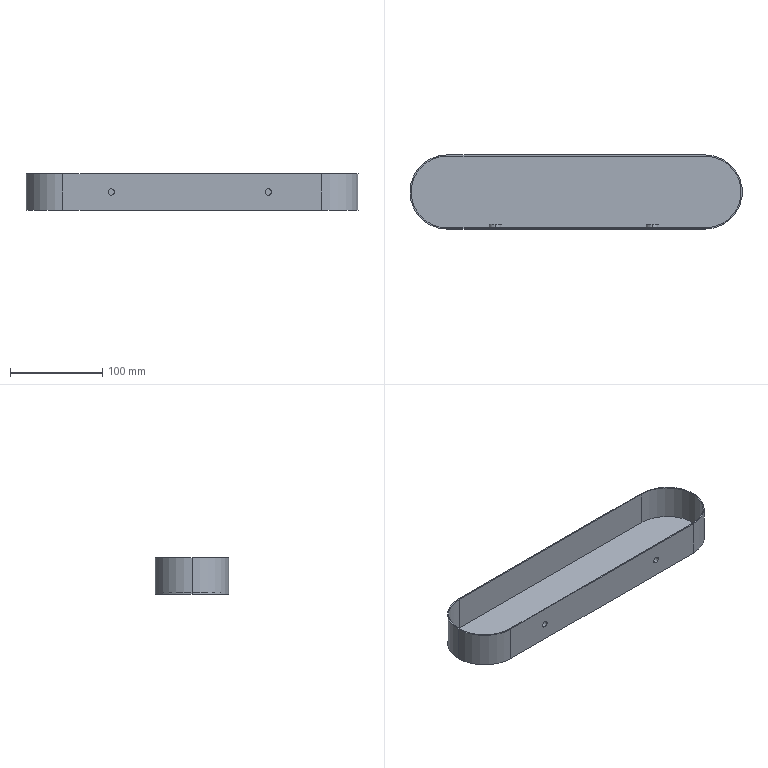Part | STEP file | 1.6米Belt罩 | 1 solid | 23 faces | box 359.4 x 80 x 39 mm | volume 70115 mm3 | cylinder 14 | plane 9 | commonest cylinder face diameters 6.8 x4 13 x4 77.6 x3 80 x3
STEP:
#1=CARTESIAN_POINT('',(222.2,-34.8,16.1));
#2=VERTEX_POINT('',#1);
#3=CARTESIAN_POINT('',(222.2,-34.8,22.9));
#4=VERTEX_POINT('',#3);
#5=CARTESIAN_POINT('',(222.2,-34.8,19.5));
#6=DIRECTION('',(0.,1.,0.));
#7=DIRECTION('',(0.,0.,1.));
#8=AXIS2_PLACEMENT_3D('',#5,#6,#7);
#9=CIRCLE('',#8,3.4);
#10=EDGE_CURVE('',#2,#4,#9,.T.);
#11=ORIENTED_EDGE('',*,*,#10,.T.);
#12=CARTESIAN_POINT('',(222.2,-40.,22.9));
#13=VERTEX_POINT('',#12);
#14=CARTESIAN_POINT('',(222.2,-40.,22.9));
#15=DIRECTION('',(0.,-1.,0.));
#16=VECTOR('',#15,1000.);
#17=LINE('',#14,#16);
#18=EDGE_CURVE('',#4,#13,#17,.T.);
#19=ORIENTED_EDGE('',*,*,#18,.T.);
#20=CARTESIAN_POINT('',(222.2,-40.,16.1));
#21=VERTEX_POINT('',#20);
#22=CARTESIAN_POINT('',(222.2,-40.,19.5));
#23=DIRECTION('',(0.,-1.,0.));
#24=DIRECTION('',(0.,0.,-1.));
#25=AXIS2_PLACEMENT_3D('',#22,#23,#24);
#26=CIRCLE('',#25,3.4);
#27=EDGE_CURVE('',#13,#21,#26,.T.);
#28=ORIENTED_EDGE('',*,*,#27,.T.);
#29=CARTESIAN_POINT('',(222.2,-40.,16.1));
#30=DIRECTION('',(0.,-1.,0.));
#31=VECTOR('',#30,1000.);
#32=LINE('',#29,#31);
#33=EDGE_CURVE('',#2,#21,#32,.T.);
#34=ORIENTED_EDGE('',*,*,#33,.F.);
#35=EDGE_LOOP('',(#11,#19,#28,#34));
#36=FACE_OUTER_BOUND('',#35,.T.);
#37=CARTESIAN_POINT('',(222.2,-40.,19.5));
#38=DIRECTION('',(0.,-1.,0.));
#39=DIRECTION('',(0.,0.,-1.));
#40=AXIS2_PLACEMENT_3D('',#37,#38,#39);
#41=CYLINDRICAL_SURFACE('',#40,3.4);
#42=ADVANCED_FACE('',(#36),#41,.F.);
#43=CARTESIAN_POINT('',(52.2,-34.8,16.1));
#44=VERTEX_POINT('',#43);
#45=CARTESIAN_POINT('',(52.2,-34.8,22.9));
#46=VERTEX_POINT('',#45);
#47=CARTESIAN_POINT('',(52.2,-34.8,19.5));
#48=DIRECTION('',(0.,1.,0.));
#49=DIRECTION('',(0.,0.,1.));
#50=AXIS2_PLACEMENT_3D('',#47,#48,#49);
#51=CIRCLE('',#50,3.4);
#52=EDGE_CURVE('',#44,#46,#51,.T.);
#53=ORIENTED_EDGE('',*,*,#52,.T.);
#54=CARTESIAN_POINT('',(52.2,-40.,22.9));
#55=VERTEX_POINT('',#54);
#56=CARTESIAN_POINT('',(52.2,-40.,22.9));
#57=DIRECTION('',(0.,-1.,0.));
#58=VECTOR('',#57,1000.);
#59=LINE('',#56,#58);
#60=EDGE_CURVE('',#46,#55,#59,.T.);
#61=ORIENTED_EDGE('',*,*,#60,.T.);
#62=CARTESIAN_POINT('',(52.2,-40.,16.1));
#63=VERTEX_POINT('',#62);
#64=CARTESIAN_POINT('',(52.2,-40.,19.5));
#65=DIRECTION('',(0.,-1.,0.));
#66=DIRECTION('',(0.,0.,-1.));
#67=AXIS2_PLACEMENT_3D('',#64,#65,#66);
#68=CIRCLE('',#67,3.4);
#69=EDGE_CURVE('',#55,#63,#68,.T.);
#70=ORIENTED_EDGE('',*,*,#69,.T.);
#71=CARTESIAN_POINT('',(52.2,-40.,16.1));
#72=DIRECTION('',(0.,-1.,0.));
#73=VECTOR('',#72,1000.);
#74=LINE('',#71,#73);
#75=EDGE_CURVE('',#44,#63,#74,.T.);
#76=ORIENTED_EDGE('',*,*,#75,.F.);
#77=EDGE_LOOP('',(#53,#61,#70,#76));
#78=FACE_OUTER_BOUND('',#77,.T.);
#79=CARTESIAN_POINT('',(52.2,-40.,19.5));
#80=DIRECTION('',(0.,-1.,0.));
#81=DIRECTION('',(0.,0.,-1.));
#82=AXIS2_PLACEMENT_3D('',#79,#80,#81);
#83=CYLINDRICAL_SURFACE('',#82,3.4);
#84=ADVANCED_FACE('',(#78),#83,.F.);
#85=CARTESIAN_POINT('',(222.2,-34.8,26.));
#86=VERTEX_POINT('',#85);
#87=CARTESIAN_POINT('',(222.2,-34.8,13.));
#88=VERTEX_POINT('',#87);
#89=CARTESIAN_POINT('',(222.2,-34.8,19.5));
#90=DIRECTION('',(0.,1.,0.));
#91=DIRECTION('',(0.,0.,1.));
#92=AXIS2_PLACEMENT_3D('',#89,#90,#91);
#93=CIRCLE('',#92,6.5);
#94=EDGE_CURVE('',#86,#88,#93,.T.);
#95=ORIENTED_EDGE('',*,*,#94,.F.);
#96=CARTESIAN_POINT('',(222.2,-38.8,26.));
#97=VERTEX_POINT('',#96);
#98=CARTESIAN_POINT('',(222.2,-34.8,26.));
#99=DIRECTION('',(0.,-1.,0.));
#100=VECTOR('',#99,1000.);
#101=LINE('',#98,#100);
#102=EDGE_CURVE('',#86,#97,#101,.T.);
#103=ORIENTED_EDGE('',*,*,#102,.T.);
#104=CARTESIAN_POINT('',(222.2,-38.8,13.));
#105=VERTEX_POINT('',#104);
#106=CARTESIAN_POINT('',(222.2,-38.8,19.5));
#107=DIRECTION('',(0.,1.,0.));
#108=DIRECTION('',(0.,0.,1.));
#109=AXIS2_PLACEMENT_3D('',#106,#107,#108);
#110=CIRCLE('',#109,6.5);
#111=EDGE_CURVE('',#97,#105,#110,.T.);
#112=ORIENTED_EDGE('',*,*,#111,.T.);
#113=CARTESIAN_POINT('',(222.2,-34.8,13.));
#114=DIRECTION('',(0.,-1.,0.));
#115=VECTOR('',#114,1000.);
#116=LINE('',#113,#115);
#117=EDGE_CURVE('',#88,#105,#116,.T.);
#118=ORIENTED_EDGE('',*,*,#117,.F.);
#119=EDGE_LOOP('',(#95,#103,#112,#118));
#120=FACE_OUTER_BOUND('',#119,.T.);
#121=CARTESIAN_POINT('',(222.2,-34.8,19.5));
#122=DIRECTION('',(0.,-1.,0.));
#123=DIRECTION('',(0.,0.,-1.));
#124=AXIS2_PLACEMENT_3D('',#121,#122,#123);
#125=CYLINDRICAL_SURFACE('',#124,6.5);
#126=ADVANCED_FACE('',(#120),#125,.T.);
#127=CARTESIAN_POINT('',(52.2,-34.8,26.));
#128=VERTEX_POINT('',#127);
#129=CARTESIAN_POINT('',(52.2,-34.8,13.));
#130=VERTEX_POINT('',#129);
#131=CARTESIAN_POINT('',(52.2,-34.8,19.5));
#132=DIRECTION('',(0.,1.,0.));
#133=DIRECTION('',(0.,0.,1.));
#134=AXIS2_PLACEMENT_3D('',#131,#132,#133);
#135=CIRCLE('',#134,6.5);
#136=EDGE_CURVE('',#128,#130,#135,.T.);
#137=ORIENTED_EDGE('',*,*,#136,.F.);
#138=CARTESIAN_POINT('',(52.2,-38.8,26.));
#139=VERTEX_POINT('',#138);
#140=CARTESIAN_POINT('',(52.2,-34.8,26.));
#141=DIRECTION('',(0.,-1.,0.));
#142=VECTOR('',#141,1000.);
#143=LINE('',#140,#142);
#144=EDGE_CURVE('',#128,#139,#143,.T.);
#145=ORIENTED_EDGE('',*,*,#144,.T.);
#146=CARTESIAN_POINT('',(52.2,-38.8,13.));
#147=VERTEX_POINT('',#146);
#148=CARTESIAN_POINT('',(52.2,-38.8,19.5));
#149=DIRECTION('',(0.,1.,0.));
#150=DIRECTION('',(0.,0.,1.));
#151=AXIS2_PLACEMENT_3D('',#148,#149,#150);
#152=CIRCLE('',#151,6.5);
#153=EDGE_CURVE('',#139,#147,#152,.T.);
#154=ORIENTED_EDGE('',*,*,#153,.T.);
#155=CARTESIAN_POINT('',(52.2,-34.8,13.));
#156=DIRECTION('',(0.,-1.,0.));
#157=VECTOR('',#156,1000.);
#158=LINE('',#155,#157);
#159=EDGE_CURVE('',#130,#147,#158,.T.);
#160=ORIENTED_EDGE('',*,*,#159,.F.);
#161=EDGE_LOOP('',(#137,#145,#154,#160));
#162=FACE_OUTER_BOUND('',#161,.T.);
#163=CARTESIAN_POINT('',(52.2,-34.8,19.5));
#164=DIRECTION('',(0.,-1.,0.));
#165=DIRECTION('',(0.,0.,-1.));
#166=AXIS2_PLACEMENT_3D('',#163,#164,#165);
#167=CYLINDRICAL_SURFACE('',#166,6.5);
#168=ADVANCED_FACE('',(#162),#167,.T.);
#169=CARTESIAN_POINT('',(0.,38.8,39.));
#170=VERTEX_POINT('',#169);
#171=CARTESIAN_POINT('',(-38.8,0.,39.));
#172=VERTEX_POINT('',#171);
#173=CARTESIAN_POINT('',(0.,0.,39.));
#174=DIRECTION('',(0.,0.,1.));
#175=DIRECTION('',(1.,0.,0.));
#176=AXIS2_PLACEMENT_3D('',#173,#174,#175);
#177=CIRCLE('',#176,38.8);
#178=EDGE_CURVE('',#170,#172,#177,.T.);
#179=ORIENTED_EDGE('',*,*,#178,.T.);
#180=CARTESIAN_POINT('',(-38.8,0.,1.2));
#181=VERTEX_POINT('',#180);
#182=CARTESIAN_POINT('',(-38.8,0.,39.));
#183=DIRECTION('',(0.,0.,-1.));
#184=VECTOR('',#183,1000.);
#185=LINE('',#182,#184);
#186=EDGE_CURVE('',#172,#181,#185,.T.);
#187=ORIENTED_EDGE('',*,*,#186,.T.);
#188=CARTESIAN_POINT('',(0.,38.8,1.2));
#189=VERTEX_POINT('',#188);
#190=CARTESIAN_POINT('',(0.,0.,1.2));
#191=DIRECTION('',(0.,0.,1.));
#192=DIRECTION('',(1.,0.,0.));
#193=AXIS2_PLACEMENT_3D('',#190,#191,#192);
#194=CIRCLE('',#193,38.8);
#195=EDGE_CURVE('',#189,#181,#194,.T.);
#196=ORIENTED_EDGE('',*,*,#195,.F.);
#197=CARTESIAN_POINT('',(0.,38.8,39.));
#198=DIRECTION('',(0.,0.,-1.));
#199=VECTOR('',#198,1000.);
#200=LINE('',#197,#199);
#201=EDGE_CURVE('',#170,#189,#200,.T.);
#202=ORIENTED_EDGE('',*,*,#201,.F.);
#203=EDGE_LOOP('',(#179,#187,#196,#202));
#204=FACE_OUTER_BOUND('',#203,.T.);
#205=CARTESIAN_POINT('',(0.,0.,39.));
#206=DIRECTION('',(0.,0.,-1.));
#207=DIRECTION('',(-1.,0.,0.));
#208=AXIS2_PLACEMENT_3D('',#205,#206,#207);
#209=CYLINDRICAL_SURFACE('',#208,38.8);
#210=ADVANCED_FACE('',(#204),#209,.F.);
#211=CARTESIAN_POINT('',(-40.,0.,39.));
#212=VERTEX_POINT('',#211);
#213=CARTESIAN_POINT('',(0.,-40.,39.));
#214=VERTEX_POINT('',#213);
#215=CARTESIAN_POINT('',(0.,0.,39.));
#216=DIRECTION('',(0.,0.,1.));
#217=DIRECTION('',(1.,0.,0.));
#218=AXIS2_PLACEMENT_3D('',#215,#216,#217);
#219=CIRCLE('',#218,40.);
#220=EDGE_CURVE('',#212,#214,#219,.T.);
#221=ORIENTED_EDGE('',*,*,#220,.F.);
#222=CARTESIAN_POINT('',(-40.,0.,0.));
#223=VERTEX_POINT('',#222);
#224=CARTESIAN_POINT('',(-40.,0.,39.));
#225=DIRECTION('',(0.,0.,-1.));
#226=VECTOR('',#225,1000.);
#227=LINE('',#224,#226);
#228=EDGE_CURVE('',#212,#223,#227,.T.);
#229=ORIENTED_EDGE('',*,*,#228,.T.);
#230=CARTESIAN_POINT('',(0.,-40.,0.));
#231=VERTEX_POINT('',#230);
#232=CARTESIAN_POINT('',(0.,0.,0.));
#233=DIRECTION('',(0.,0.,1.));
#234=DIRECTION('',(1.,0.,0.));
#235=AXIS2_PLACEMENT_3D('',#232,#233,#234);
#236=CIRCLE('',#235,40.);
#237=EDGE_CURVE('',#223,#231,#236,.T.);
#238=ORIENTED_EDGE('',*,*,#237,.T.);
#239=CARTESIAN_POINT('',(0.,-40.,39.));
#240=DIRECTION('',(0.,0.,-1.));
#241=VECTOR('',#240,1000.);
#242=LINE('',#239,#241);
#243=EDGE_CURVE('',#214,#231,#242,.T.);
#244=ORIENTED_EDGE('',*,*,#243,.F.);
#245=EDGE_LOOP('',(#221,#229,#238,#244));
#246=FACE_OUTER_BOUND('',#245,.T.);
#247=CARTESIAN_POINT('',(0.,0.,39.));
#248=DIRECTION('',(0.,0.,-1.));
#249=DIRECTION('',(-1.,0.,0.));
#250=AXIS2_PLACEMENT_3D('',#247,#248,#249);
#251=CYLINDRICAL_SURFACE('',#250,40.);
#252=ADVANCED_FACE('',(#246),#251,.T.);
#253=ORIENTED_EDGE('',*,*,#228,.F.);
#254=CARTESIAN_POINT('',(0.,40.,39.));
#255=VERTEX_POINT('',#254);
#256=CARTESIAN_POINT('',(0.,0.,39.));
#257=DIRECTION('',(0.,0.,1.));
#258=DIRECTION('',(1.,0.,0.));
#259=AXIS2_PLACEMENT_3D('',#256,#257,#258);
#260=CIRCLE('',#259,40.);
#261=EDGE_CURVE('',#255,#212,#260,.T.);
#262=ORIENTED_EDGE('',*,*,#261,.F.);
#263=CARTESIAN_POINT('',(0.,40.,0.));
#264=VERTEX_POINT('',#263);
#265=CARTESIAN_POINT('',(0.,40.,39.));
#266=DIRECTION('',(0.,0.,-1.));
#267=VECTOR('',#266,1000.);
#268=LINE('',#265,#267);
#269=EDGE_CURVE('',#255,#264,#268,.T.);
#270=ORIENTED_EDGE('',*,*,#269,.T.);
#271=CARTESIAN_POINT('',(0.,0.,0.));
#272=DIRECTION('',(0.,0.,1.));
#273=DIRECTION('',(1.,0.,0.));
#274=AXIS2_PLACEMENT_3D('',#271,#272,#273);
#275=CIRCLE('',#274,40.);
#276=EDGE_CURVE('',#264,#223,#275,.T.);
#277=ORIENTED_EDGE('',*,*,#276,.T.);
#278=EDGE_LOOP('',(#253,#262,#270,#277));
#279=FACE_OUTER_BOUND('',#278,.T.);
#280=CARTESIAN_POINT('',(0.,0.,39.));
#281=DIRECTION('',(0.,0.,-1.));
#282=DIRECTION('',(-1.,0.,0.));
#283=AXIS2_PLACEMENT_3D('',#280,#281,#282);
#284=CYLINDRICAL_SURFACE('',#283,40.);
#285=ADVANCED_FACE('',(#279),#284,.T.);
#286=CARTESIAN_POINT('',(222.2,-40.,19.5));
#287=DIRECTION('',(0.,-1.,0.));
#288=DIRECTION('',(0.,0.,-1.));
#289=AXIS2_PLACEMENT_3D('',#286,#287,#288);
#290=CIRCLE('',#289,3.4);
#291=EDGE_CURVE('',#21,#13,#290,.T.);
#292=ORIENTED_EDGE('',*,*,#291,.F.);
#293=ORIENTED_EDGE('',*,*,#27,.F.);
#294=EDGE_LOOP('',(#292,#293));
#295=FACE_BOUND('',#294,.T.);
#296=CARTESIAN_POINT('',(52.2,-40.,19.5));
#297=DIRECTION('',(0.,-1.,0.));
#298=DIRECTION('',(0.,0.,-1.));
#299=AXIS2_PLACEMENT_3D('',#296,#297,#298);
#300=CIRCLE('',#299,3.4);
#301=EDGE_CURVE('',#63,#55,#300,.T.);
#302=ORIENTED_EDGE('',*,*,#301,.F.);
#303=ORIENTED_EDGE('',*,*,#69,.F.);
#304=EDGE_LOOP('',(#302,#303));
#305=FACE_BOUND('',#304,.T.);
#306=CARTESIAN_POINT('',(279.4,-40.,0.));
#307=VERTEX_POINT('',#306);
#308=CARTESIAN_POINT('',(0.,-40.,0.));
#309=DIRECTION('',(1.,0.,0.));
#310=VECTOR('',#309,1000.);
#311=LINE('',#308,#310);
#312=EDGE_CURVE('',#231,#307,#311,.T.);
#313=ORIENTED_EDGE('',*,*,#312,.T.);
#314=CARTESIAN_POINT('',(279.4,-40.,39.));
#315=VERTEX_POINT('',#314);
#316=CARTESIAN_POINT('',(279.4,-40.,39.));
#317=DIRECTION('',(0.,0.,-1.));
#318=VECTOR('',#317,1000.);
#319=LINE('',#316,#318);
#320=EDGE_CURVE('',#315,#307,#319,.T.);
#321=ORIENTED_EDGE('',*,*,#320,.F.);
#322=CARTESIAN_POINT('',(0.,-40.,39.));
#323=DIRECTION('',(1.,0.,0.));
#324=VECTOR('',#323,1000.);
#325=LINE('',#322,#324);
#326=EDGE_CURVE('',#214,#315,#325,.T.);
#327=ORIENTED_EDGE('',*,*,#326,.F.);
#328=ORIENTED_EDGE('',*,*,#243,.T.);
#329=EDGE_LOOP('',(#313,#321,#327,#328));
#330=FACE_OUTER_BOUND('',#329,.T.);
#331=CARTESIAN_POINT('',(0.,-40.,39.));
#332=DIRECTION('',(0.,1.,0.));
#333=DIRECTION('',(0.,0.,1.));
#334=AXIS2_PLACEMENT_3D('',#331,#332,#333);
#335=PLANE('',#334);
#336=ADVANCED_FACE('',(#295,#305,#330),#335,.F.);
#337=CARTESIAN_POINT('',(279.4,40.,0.));
#338=VERTEX_POINT('',#337);
#339=CARTESIAN_POINT('',(279.4,0.,0.));
#340=DIRECTION('',(0.,0.,1.));
#341=DIRECTION('',(1.,0.,0.));
#342=AXIS2_PLACEMENT_3D('',#339,#340,#341);
#343=CIRCLE('',#342,40.);
#344=EDGE_CURVE('',#307,#338,#343,.T.);
#345=ORIENTED_EDGE('',*,*,#344,.T.);
#346=CARTESIAN_POINT('',(279.4,40.,39.));
#347=VERTEX_POINT('',#346);
#348=CARTESIAN_POINT('',(279.4,40.,39.));
#349=DIRECTION('',(0.,0.,-1.));
#350=VECTOR('',#349,1000.);
#351=LINE('',#348,#350);
#352=EDGE_CURVE('',#347,#338,#351,.T.);
#353=ORIENTED_EDGE('',*,*,#352,.F.);
#354=CARTESIAN_POINT('',(279.4,0.,39.));
#355=DIRECTION('',(0.,0.,1.));
#356=DIRECTION('',(1.,0.,0.));
#357=AXIS2_PLACEMENT_3D('',#354,#355,#356);
#358=CIRCLE('',#357,40.);
#359=EDGE_CURVE('',#315,#347,#358,.T.);
#360=ORIENTED_EDGE('',*,*,#359,.F.);
#361=ORIENTED_EDGE('',*,*,#320,.T.);
#362=EDGE_LOOP('',(#345,#353,#360,#361));
#363=FACE_OUTER_BOUND('',#362,.T.);
#364=CARTESIAN_POINT('',(279.4,0.,39.));
#365=DIRECTION('',(0.,0.,-1.));
#366=DIRECTION('',(-1.,0.,0.));
#367=AXIS2_PLACEMENT_3D('',#364,#365,#366);
#368=CYLINDRICAL_SURFACE('',#367,40.);
#369=ADVANCED_FACE('',(#363),#368,.T.);
#370=CARTESIAN_POINT('',(0.,40.,0.));
#371=DIRECTION('',(-1.,0.,0.));
#372=VECTOR('',#371,1000.);
#373=LINE('',#370,#372);
#374=EDGE_CURVE('',#338,#264,#373,.T.);
#375=ORIENTED_EDGE('',*,*,#374,.T.);
#376=ORIENTED_EDGE('',*,*,#269,.F.);
#377=CARTESIAN_POINT('',(0.,40.,39.));
#378=DIRECTION('',(-1.,0.,0.));
#379=VECTOR('',#378,1000.);
#380=LINE('',#377,#379);
#381=EDGE_CURVE('',#347,#255,#380,.T.);
#382=ORIENTED_EDGE('',*,*,#381,.F.);
#383=ORIENTED_EDGE('',*,*,#352,.T.);
#384=EDGE_LOOP('',(#375,#376,#382,#383));
#385=FACE_OUTER_BOUND('',#384,.T.);
#386=CARTESIAN_POINT('',(0.,40.,39.));
#387=DIRECTION('',(0.,-1.,0.));
#388=DIRECTION('',(0.,0.,-1.));
#389=AXIS2_PLACEMENT_3D('',#386,#387,#388);
#390=PLANE('',#389);
#391=ADVANCED_FACE('',(#385),#390,.F.);
#392=ORIENTED_EDGE('',*,*,#178,.F.);
#393=CARTESIAN_POINT('',(279.4,38.8,39.));
#394=VERTEX_POINT('',#393);
#395=CARTESIAN_POINT('',(0.,38.8,39.));
#396=DIRECTION('',(-1.,0.,0.));
#397=VECTOR('',#396,1000.);
#398=LINE('',#395,#397);
#399=EDGE_CURVE('',#394,#170,#398,.T.);
#400=ORIENTED_EDGE('',*,*,#399,.F.);
#401=CARTESIAN_POINT('',(279.4,-38.8,39.));
#402=VERTEX_POINT('',#401);
#403=CARTESIAN_POINT('',(279.4,0.,39.));
#404=DIRECTION('',(0.,0.,1.));
#405=DIRECTION('',(1.,0.,0.));
#406=AXIS2_PLACEMENT_3D('',#403,#404,#405);
#407=CIRCLE('',#406,38.8);
#408=EDGE_CURVE('',#402,#394,#407,.T.);
#409=ORIENTED_EDGE('',*,*,#408,.F.);
#410=CARTESIAN_POINT('',(0.,-38.8,39.));
#411=VERTEX_POINT('',#410);
#412=CARTESIAN_POINT('',(0.,-38.8,39.));
#413=DIRECTION('',(1.,0.,0.));
#414=VECTOR('',#413,1000.);
#415=LINE('',#412,#414);
#416=EDGE_CURVE('',#411,#402,#415,.T.);
#417=ORIENTED_EDGE('',*,*,#416,.F.);
#418=CARTESIAN_POINT('',(0.,0.,39.));
#419=DIRECTION('',(0.,0.,1.));
#420=DIRECTION('',(1.,0.,0.));
#421=AXIS2_PLACEMENT_3D('',#418,#419,#420);
#422=CIRCLE('',#421,38.8);
#423=EDGE_CURVE('',#172,#411,#422,.T.);
#424=ORIENTED_EDGE('',*,*,#423,.F.);
#425=EDGE_LOOP('',(#392,#400,#409,#417,#424));
#426=FACE_BOUND('',#425,.T.);
#427=ORIENTED_EDGE('',*,*,#261,.T.);
#428=ORIENTED_EDGE('',*,*,#220,.T.);
#429=ORIENTED_EDGE('',*,*,#326,.T.);
#430=ORIENTED_EDGE('',*,*,#359,.T.);
#431=ORIENTED_EDGE('',*,*,#381,.T.);
#432=EDGE_LOOP('',(#427,#428,#429,#430,#431));
#433=FACE_OUTER_BOUND('',#432,.T.);
#434=CARTESIAN_POINT('',(0.,0.,39.));
#435=DIRECTION('',(0.,0.,1.));
#436=DIRECTION('',(1.,0.,0.));
#437=AXIS2_PLACEMENT_3D('',#434,#435,#436);
#438=PLANE('',#437);
#439=ADVANCED_FACE('',(#426,#433),#438,.T.);
#440=ORIENTED_EDGE('',*,*,#276,.F.);
#441=ORIENTED_EDGE('',*,*,#374,.F.);
#442=ORIENTED_EDGE('',*,*,#344,.F.);
#443=ORIENTED_EDGE('',*,*,#312,.F.);
#444=ORIENTED_EDGE('',*,*,#237,.F.);
#445=EDGE_LOOP('',(#440,#441,#442,#443,#444));
#446=FACE_OUTER_BOUND('',#445,.T.);
#447=CARTESIAN_POINT('',(0.,0.,0.));
#448=DIRECTION('',(0.,0.,1.));
#449=DIRECTION('',(1.,0.,0.));
#450=AXIS2_PLACEMENT_3D('',#447,#448,#449);
#451=PLANE('',#450);
#452=ADVANCED_FACE('',(#446),#451,.F.);
#453=ORIENTED_EDGE('',*,*,#186,.F.);
#454=ORIENTED_EDGE('',*,*,#423,.T.);
#455=CARTESIAN_POINT('',(0.,-38.8,1.2));
#456=VERTEX_POINT('',#455);
#457=CARTESIAN_POINT('',(0.,-38.8,39.));
#458=DIRECTION('',(0.,0.,-1.));
#459=VECTOR('',#458,1000.);
#460=LINE('',#457,#459);
#461=EDGE_CURVE('',#411,#456,#460,.T.);
#462=ORIENTED_EDGE('',*,*,#461,.T.);
#463=CARTESIAN_POINT('',(0.,0.,1.2));
#464=DIRECTION('',(0.,0.,1.));
#465=DIRECTION('',(1.,0.,0.));
#466=AXIS2_PLACEMENT_3D('',#463,#464,#465);
#467=CIRCLE('',#466,38.8);
#468=EDGE_CURVE('',#181,#456,#467,.T.);
#469=ORIENTED_EDGE('',*,*,#468,.F.);
#470=EDGE_LOOP('',(#453,#454,#462,#469));
#471=FACE_OUTER_BOUND('',#470,.T.);
#472=CARTESIAN_POINT('',(0.,0.,39.));
#473=DIRECTION('',(0.,0.,-1.));
#474=DIRECTION('',(-1.,0.,0.));
#475=AXIS2_PLACEMENT_3D('',#472,#473,#474);
#476=CYLINDRICAL_SURFACE('',#475,38.8);
#477=ADVANCED_FACE('',(#471),#476,.F.);
#478=CARTESIAN_POINT('',(222.2,-38.8,19.5));
#479=DIRECTION('',(0.,1.,0.));
#480=DIRECTION('',(0.,0.,1.));
#481=AXIS2_PLACEMENT_3D('',#478,#479,#480);
#482=CIRCLE('',#481,6.5);
#483=EDGE_CURVE('',#105,#97,#482,.T.);
#484=ORIENTED_EDGE('',*,*,#483,.F.);
#485=ORIENTED_EDGE('',*,*,#111,.F.);
#486=EDGE_LOOP('',(#484,#485));
#487=FACE_BOUND('',#486,.T.);
#488=CARTESIAN_POINT('',(52.2,-38.8,19.5));
#489=DIRECTION('',(0.,1.,0.));
#490=DIRECTION('',(0.,0.,1.));
#491=AXIS2_PLACEMENT_3D('',#488,#489,#490);
#492=CIRCLE('',#491,6.5);
#493=EDGE_CURVE('',#147,#139,#492,.T.);
#494=ORIENTED_EDGE('',*,*,#493,.F.);
#495=ORIENTED_EDGE('',*,*,#153,.F.);
#496=EDGE_LOOP('',(#494,#495));
#497=FACE_BOUND('',#496,.T.);
#498=CARTESIAN_POINT('',(279.4,-38.8,1.2));
#499=VERTEX_POINT('',#498);
#500=CARTESIAN_POINT('',(0.,-38.8,1.2));
#501=DIRECTION('',(1.,0.,0.));
#502=VECTOR('',#501,1000.);
#503=LINE('',#500,#502);
#504=EDGE_CURVE('',#456,#499,#503,.T.);
#505=ORIENTED_EDGE('',*,*,#504,.F.);
#506=ORIENTED_EDGE('',*,*,#461,.F.);
#507=ORIENTED_EDGE('',*,*,#416,.T.);
#508=CARTESIAN_POINT('',(279.4,-38.8,39.));
#509=DIRECTION('',(0.,0.,-1.));
#510=VECTOR('',#509,1000.);
#511=LINE('',#508,#510);
#512=EDGE_CURVE('',#402,#499,#511,.T.);
#513=ORIENTED_EDGE('',*,*,#512,.T.);
#514=EDGE_LOOP('',(#505,#506,#507,#513));
#515=FACE_OUTER_BOUND('',#514,.T.);
#516=CARTESIAN_POINT('',(0.,-38.8,39.));
#517=DIRECTION('',(0.,1.,0.));
#518=DIRECTION('',(0.,0.,1.));
#519=AXIS2_PLACEMENT_3D('',#516,#517,#518);
#520=PLANE('',#519);
#521=ADVANCED_FACE('',(#487,#497,#515),#520,.T.);
#522=CARTESIAN_POINT('',(279.4,38.8,1.2));
#523=VERTEX_POINT('',#522);
#524=CARTESIAN_POINT('',(279.4,0.,1.2));
#525=DIRECTION('',(0.,0.,1.));
#526=DIRECTION('',(1.,0.,0.));
#527=AXIS2_PLACEMENT_3D('',#524,#525,#526);
#528=CIRCLE('',#527,38.8);
#529=EDGE_CURVE('',#499,#523,#528,.T.);
#530=ORIENTED_EDGE('',*,*,#529,.F.);
#531=ORIENTED_EDGE('',*,*,#512,.F.);
#532=ORIENTED_EDGE('',*,*,#408,.T.);
#533=CARTESIAN_POINT('',(279.4,38.8,39.));
#534=DIRECTION('',(0.,0.,-1.));
#535=VECTOR('',#534,1000.);
#536=LINE('',#533,#535);
#537=EDGE_CURVE('',#394,#523,#536,.T.);
#538=ORIENTED_EDGE('',*,*,#537,.T.);
#539=EDGE_LOOP('',(#530,#531,#532,#538));
#540=FACE_OUTER_BOUND('',#539,.T.);
#541=CARTESIAN_POINT('',(279.4,0.,39.));
#542=DIRECTION('',(0.,0.,-1.));
#543=DIRECTION('',(-1.,0.,0.));
#544=AXIS2_PLACEMENT_3D('',#541,#542,#543);
#545=CYLINDRICAL_SURFACE('',#544,38.8);
#546=ADVANCED_FACE('',(#540),#545,.F.);
#547=CARTESIAN_POINT('',(0.,38.8,1.2));
#548=DIRECTION('',(-1.,0.,0.));
#549=VECTOR('',#548,1000.);
#550=LINE('',#547,#549);
#551=EDGE_CURVE('',#523,#189,#550,.T.);
#552=ORIENTED_EDGE('',*,*,#551,.F.);
#553=ORIENTED_EDGE('',*,*,#537,.F.);
#554=ORIENTED_EDGE('',*,*,#399,.T.);
#555=ORIENTED_EDGE('',*,*,#201,.T.);
#556=EDGE_LOOP('',(#552,#553,#554,#555));
#557=FACE_OUTER_BOUND('',#556,.T.);
#558=CARTESIAN_POINT('',(0.,38.8,39.));
#559=DIRECTION('',(0.,-1.,0.));
#560=DIRECTION('',(0.,0.,-1.));
#561=AXIS2_PLACEMENT_3D('',#558,#559,#560);
#562=PLANE('',#561);
#563=ADVANCED_FACE('',(#557),#562,.T.);
#564=ORIENTED_EDGE('',*,*,#195,.T.);
#565=ORIENTED_EDGE('',*,*,#468,.T.);
#566=ORIENTED_EDGE('',*,*,#504,.T.);
#567=ORIENTED_EDGE('',*,*,#529,.T.);
#568=ORIENTED_EDGE('',*,*,#551,.T.);
#569=EDGE_LOOP('',(#564,#565,#566,#567,#568));
#570=FACE_OUTER_BOUND('',#569,.T.);
#571=CARTESIAN_POINT('',(0.,0.,1.2));
#572=DIRECTION('',(0.,0.,1.));
#573=DIRECTION('',(1.,0.,0.));
#574=AXIS2_PLACEMENT_3D('',#571,#572,#573);
#575=PLANE('',#574);
#576=ADVANCED_FACE('',(#570),#575,.T.);
#577=ORIENTED_EDGE('',*,*,#144,.F.);
#578=CARTESIAN_POINT('',(52.2,-34.8,19.5));
#579=DIRECTION('',(0.,1.,0.));
#580=DIRECTION('',(0.,0.,1.));
#581=AXIS2_PLACEMENT_3D('',#578,#579,#580);
#582=CIRCLE('',#581,6.5);
#583=EDGE_CURVE('',#130,#128,#582,.T.);
#584=ORIENTED_EDGE('',*,*,#583,.F.);
#585=ORIENTED_EDGE('',*,*,#159,.T.);
#586=ORIENTED_EDGE('',*,*,#493,.T.);
#587=EDGE_LOOP('',(#577,#584,#585,#586));
#588=FACE_OUTER_BOUND('',#587,.T.);
#589=CARTESIAN_POINT('',(52.2,-34.8,19.5));
#590=DIRECTION('',(0.,-1.,0.));
#591=DIRECTION('',(0.,0.,-1.));
#592=AXIS2_PLACEMENT_3D('',#589,#590,#591);
#593=CYLINDRICAL_SURFACE('',#592,6.5);
#594=ADVANCED_FACE('',(#588),#593,.T.);
#595=ORIENTED_EDGE('',*,*,#52,.F.);
#596=CARTESIAN_POINT('',(52.2,-34.8,19.5));
#597=DIRECTION('',(0.,1.,0.));
#598=DIRECTION('',(0.,0.,1.));
#599=AXIS2_PLACEMENT_3D('',#596,#597,#598);
#600=CIRCLE('',#599,3.4);
#601=EDGE_CURVE('',#46,#44,#600,.T.);
#602=ORIENTED_EDGE('',*,*,#601,.F.);
#603=EDGE_LOOP('',(#595,#602));
#604=FACE_BOUND('',#603,.T.);
#605=ORIENTED_EDGE('',*,*,#583,.T.);
#606=ORIENTED_EDGE('',*,*,#136,.T.);
#607=EDGE_LOOP('',(#605,#606));
#608=FACE_OUTER_BOUND('',#607,.T.);
#609=CARTESIAN_POINT('',(52.2,-34.8,19.5));
#610=DIRECTION('',(0.,1.,0.));
#611=DIRECTION('',(0.,0.,1.));
#612=AXIS2_PLACEMENT_3D('',#609,#610,#611);
#613=PLANE('',#612);
#614=ADVANCED_FACE('',(#604,#608),#613,.T.);
#615=ORIENTED_EDGE('',*,*,#102,.F.);
#616=CARTESIAN_POINT('',(222.2,-34.8,19.5));
#617=DIRECTION('',(0.,1.,0.));
#618=DIRECTION('',(0.,0.,1.));
#619=AXIS2_PLACEMENT_3D('',#616,#617,#618);
#620=CIRCLE('',#619,6.5);
#621=EDGE_CURVE('',#88,#86,#620,.T.);
#622=ORIENTED_EDGE('',*,*,#621,.F.);
#623=ORIENTED_EDGE('',*,*,#117,.T.);
#624=ORIENTED_EDGE('',*,*,#483,.T.);
#625=EDGE_LOOP('',(#615,#622,#623,#624));
#626=FACE_OUTER_BOUND('',#625,.T.);
#627=CARTESIAN_POINT('',(222.2,-34.8,19.5));
#628=DIRECTION('',(0.,-1.,0.));
#629=DIRECTION('',(0.,0.,-1.));
#630=AXIS2_PLACEMENT_3D('',#627,#628,#629);
#631=CYLINDRICAL_SURFACE('',#630,6.5);
#632=ADVANCED_FACE('',(#626),#631,.T.);
#633=ORIENTED_EDGE('',*,*,#10,.F.);
#634=CARTESIAN_POINT('',(222.2,-34.8,19.5));
#635=DIRECTION('',(0.,1.,0.));
#636=DIRECTION('',(0.,0.,1.));
#637=AXIS2_PLACEMENT_3D('',#634,#635,#636);
#638=CIRCLE('',#637,3.4);
#639=EDGE_CURVE('',#4,#2,#638,.T.);
#640=ORIENTED_EDGE('',*,*,#639,.F.);
#641=EDGE_LOOP('',(#633,#640));
#642=FACE_BOUND('',#641,.T.);
#643=ORIENTED_EDGE('',*,*,#621,.T.);
#644=ORIENTED_EDGE('',*,*,#94,.T.);
#645=EDGE_LOOP('',(#643,#644));
#646=FACE_OUTER_BOUND('',#645,.T.);
#647=CARTESIAN_POINT('',(222.2,-34.8,19.5));
#648=DIRECTION('',(0.,1.,0.));
#649=DIRECTION('',(0.,0.,1.));
#650=AXIS2_PLACEMENT_3D('',#647,#648,#649);
#651=PLANE('',#650);
#652=ADVANCED_FACE('',(#642,#646),#651,.T.);
#653=ORIENTED_EDGE('',*,*,#60,.F.);
#654=ORIENTED_EDGE('',*,*,#601,.T.);
#655=ORIENTED_EDGE('',*,*,#75,.T.);
#656=ORIENTED_EDGE('',*,*,#301,.T.);
#657=EDGE_LOOP('',(#653,#654,#655,#656));
#658=FACE_OUTER_BOUND('',#657,.T.);
#659=CARTESIAN_POINT('',(52.2,-40.,19.5));
#660=DIRECTION('',(0.,-1.,0.));
#661=DIRECTION('',(0.,0.,-1.));
#662=AXIS2_PLACEMENT_3D('',#659,#660,#661);
#663=CYLINDRICAL_SURFACE('',#662,3.4);
#664=ADVANCED_FACE('',(#658),#663,.F.);
#665=ORIENTED_EDGE('',*,*,#18,.F.);
#666=ORIENTED_EDGE('',*,*,#639,.T.);
#667=ORIENTED_EDGE('',*,*,#33,.T.);
#668=ORIENTED_EDGE('',*,*,#291,.T.);
#669=EDGE_LOOP('',(#665,#666,#667,#668));
#670=FACE_OUTER_BOUND('',#669,.T.);
#671=CARTESIAN_POINT('',(222.2,-40.,19.5));
#672=DIRECTION('',(0.,-1.,0.));
#673=DIRECTION('',(0.,0.,-1.));
#674=AXIS2_PLACEMENT_3D('',#671,#672,#673);
#675=CYLINDRICAL_SURFACE('',#674,3.4);
#676=ADVANCED_FACE('',(#670),#675,.F.);
#677=CLOSED_SHELL('',(#42,#84,#126,#168,#210,#252,#285,#336,#369,#391,#439,#452,#477,#521,#546,#563,#576,#594,#614,#632,#652,#664,#676));
#678=MANIFOLD_SOLID_BREP('',#677);
#679=CARTESIAN_POINT('',(0.,0.,0.));
#680=DIRECTION('',(0.,0.,1.));
#681=DIRECTION('',(1.,0.,0.));
#682=AXIS2_PLACEMENT_3D('',#679,#680,#681);
#683=(LENGTH_UNIT()NAMED_UNIT(*)SI_UNIT(.MILLI.,.METRE.));
#684=UNCERTAINTY_MEASURE_WITH_UNIT(LENGTH_MEASURE(0.00001),#683,'','');
#685=(NAMED_UNIT(*)PLANE_ANGLE_UNIT()SI_UNIT($,.RADIAN.));
#686=(NAMED_UNIT(*)SI_UNIT($,.STERADIAN.)SOLID_ANGLE_UNIT());
#687=(GEOMETRIC_REPRESENTATION_CONTEXT(3)GLOBAL_UNCERTAINTY_ASSIGNED_CONTEXT((#684))GLOBAL_UNIT_ASSIGNED_CONTEXT((#683,#685,#686))REPRESENTATION_CONTEXT('',''));
#688=ADVANCED_BREP_SHAPE_REPRESENTATION('',(#678,#682),#687);